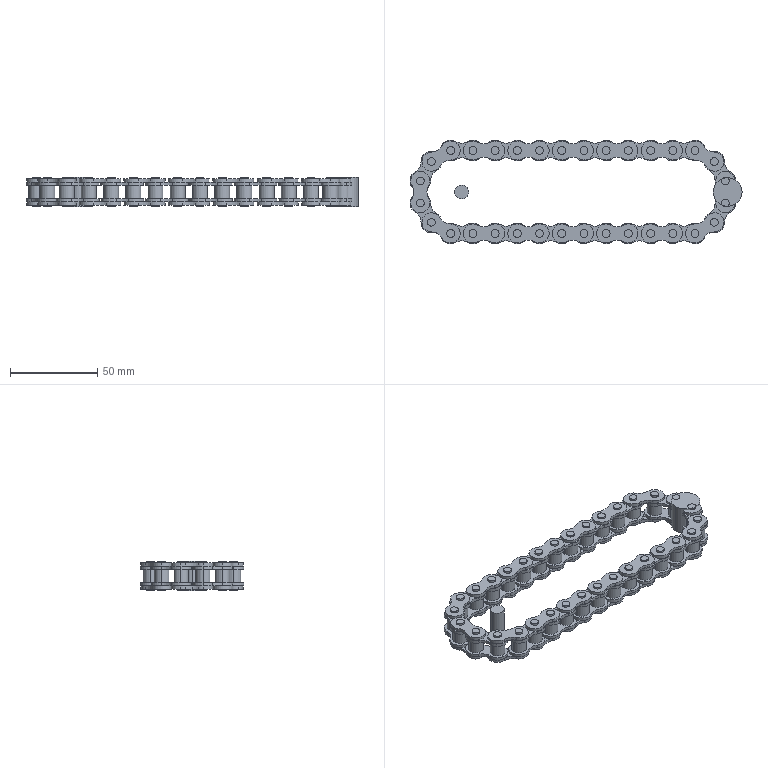Part | SolidWorks | features ICE 6, Extrusion 1, MirrorPattern 1 | 3 solids | 857 faces | box 189.793 x 59.207 x 17 mm | volume 45007 mm3 | cylinder 661 | plane 196 | commonest cylinder face diameters 4.45 x256 10.92 x108 11.81 x97 14.48 x68 8.51 x64 13.59 x64